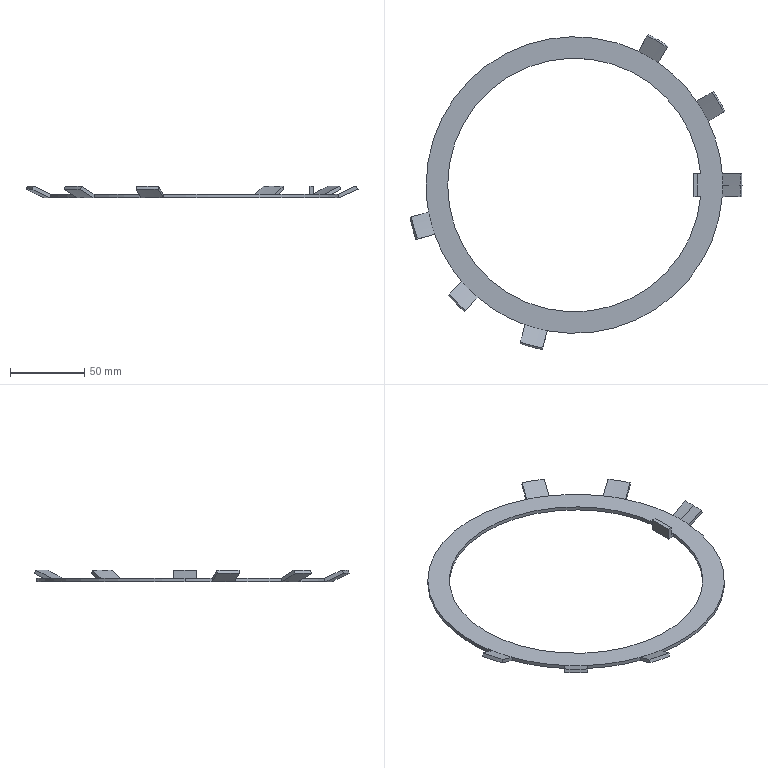Part | SolidWorks | features Boss 1, Cut 1, Revolution 1 | 1 solid | 48 faces | box 223.898 x 212.404 x 8.087 mm | volume 24578 mm3 | cone 20 | plane 19 | cylinder 9 | commonest cylinder face diameters 200 x7 171 x2
STEP:
#1=CARTESIAN_POINT('',(-100.,0.,-5.587));
#2=VERTEX_POINT('',#1);
#3=CARTESIAN_POINT('',(-98.308,-18.318,-5.587));
#4=VERTEX_POINT('',#3);
#5=CARTESIAN_POINT('',(0.,0.,-5.587));
#6=DIRECTION('',(0.,0.,1.));
#7=DIRECTION('',(1.,0.,0.));
#8=AXIS2_PLACEMENT_3D('',#5,#6,#7);
#9=CIRCLE('',#8,100.);
#10=EDGE_CURVE('',#2,#4,#9,.T.);
#11=ORIENTED_EDGE('',*,*,#10,.F.);
#12=CARTESIAN_POINT('',(-100.,0.,-8.087));
#13=VERTEX_POINT('',#12);
#14=CARTESIAN_POINT('',(-100.,0.,0.));
#15=DIRECTION('',(0.,0.,-1.));
#16=VECTOR('',#15,1000.);
#17=LINE('',#14,#16);
#18=EDGE_CURVE('',#2,#13,#17,.T.);
#19=ORIENTED_EDGE('',*,*,#18,.T.);
#20=CARTESIAN_POINT('',(-98.308,-18.318,-8.087));
#21=VERTEX_POINT('',#20);
#22=CARTESIAN_POINT('',(0.,0.,-8.087));
#23=DIRECTION('',(0.,0.,-1.));
#24=DIRECTION('',(-1.,0.,0.));
#25=AXIS2_PLACEMENT_3D('',#22,#23,#24);
#26=CIRCLE('',#25,100.);
#27=EDGE_CURVE('',#21,#13,#26,.T.);
#28=ORIENTED_EDGE('',*,*,#27,.F.);
#29=CARTESIAN_POINT('',(-98.308,-18.318,0.));
#30=DIRECTION('',(0.,0.,-1.));
#31=VECTOR('',#30,1000.);
#32=LINE('',#29,#31);
#33=EDGE_CURVE('',#4,#21,#32,.T.);
#34=ORIENTED_EDGE('',*,*,#33,.F.);
#35=EDGE_LOOP('',(#11,#19,#28,#34));
#36=FACE_OUTER_BOUND('',#35,.T.);
#37=CARTESIAN_POINT('',(0.,0.,0.));
#38=DIRECTION('',(0.,0.,-1.));
#39=DIRECTION('',(-1.,0.,0.));
#40=AXIS2_PLACEMENT_3D('',#37,#38,#39);
#41=CYLINDRICAL_SURFACE('',#40,100.);
#42=ADVANCED_FACE('',(#36),#41,.T.);
#43=CARTESIAN_POINT('',(85.148,7.75,-5.587));
#44=VERTEX_POINT('',#43);
#45=CARTESIAN_POINT('',(-85.5,0.,-5.587));
#46=VERTEX_POINT('',#45);
#47=CARTESIAN_POINT('',(0.,0.,-5.587));
#48=DIRECTION('',(0.,0.,1.));
#49=DIRECTION('',(1.,0.,0.));
#50=AXIS2_PLACEMENT_3D('',#47,#48,#49);
#51=CIRCLE('',#50,85.5);
#52=EDGE_CURVE('',#44,#46,#51,.T.);
#53=ORIENTED_EDGE('',*,*,#52,.T.);
#54=CARTESIAN_POINT('',(-85.5,0.,-8.087));
#55=VERTEX_POINT('',#54);
#56=CARTESIAN_POINT('',(-85.5,0.,0.));
#57=DIRECTION('',(0.,0.,-1.));
#58=VECTOR('',#57,1000.);
#59=LINE('',#56,#58);
#60=EDGE_CURVE('',#46,#55,#59,.T.);
#61=ORIENTED_EDGE('',*,*,#60,.T.);
#62=CARTESIAN_POINT('',(85.148,7.75,-8.087));
#63=VERTEX_POINT('',#62);
#64=CARTESIAN_POINT('',(0.,0.,-8.087));
#65=DIRECTION('',(0.,0.,-1.));
#66=DIRECTION('',(-1.,0.,0.));
#67=AXIS2_PLACEMENT_3D('',#64,#65,#66);
#68=CIRCLE('',#67,85.5);
#69=EDGE_CURVE('',#55,#63,#68,.T.);
#70=ORIENTED_EDGE('',*,*,#69,.T.);
#71=CARTESIAN_POINT('',(85.148,7.75,0.));
#72=DIRECTION('',(0.,0.,-1.));
#73=VECTOR('',#72,1000.);
#74=LINE('',#71,#73);
#75=EDGE_CURVE('',#44,#63,#74,.T.);
#76=ORIENTED_EDGE('',*,*,#75,.F.);
#77=EDGE_LOOP('',(#53,#61,#70,#76));
#78=FACE_OUTER_BOUND('',#77,.T.);
#79=CARTESIAN_POINT('',(0.,0.,0.));
#80=DIRECTION('',(0.,0.,-1.));
#81=DIRECTION('',(-1.,0.,0.));
#82=AXIS2_PLACEMENT_3D('',#79,#80,#81);
#83=CYLINDRICAL_SURFACE('',#82,85.5);
#84=ADVANCED_FACE('',(#78),#83,.F.);
#85=CARTESIAN_POINT('',(100.,0.,-5.587));
#86=VERTEX_POINT('',#85);
#87=CARTESIAN_POINT('',(99.699,7.75,-5.587));
#88=VERTEX_POINT('',#87);
#89=CARTESIAN_POINT('',(0.,0.,-5.587));
#90=DIRECTION('',(0.,0.,1.));
#91=DIRECTION('',(1.,0.,0.));
#92=AXIS2_PLACEMENT_3D('',#89,#90,#91);
#93=CIRCLE('',#92,100.);
#94=EDGE_CURVE('',#86,#88,#93,.T.);
#95=ORIENTED_EDGE('',*,*,#94,.F.);
#96=CARTESIAN_POINT('',(111.981,0.,0.));
#97=VERTEX_POINT('',#96);
#98=CARTESIAN_POINT('',(100.,0.,-5.587));
#99=DIRECTION('',(0.9063,0.,0.4226));
#100=VECTOR('',#99,1000.);
#101=LINE('',#98,#100);
#102=EDGE_CURVE('',#86,#97,#101,.T.);
#103=ORIENTED_EDGE('',*,*,#102,.T.);
#104=CARTESIAN_POINT('',(111.712,7.75,0.));
#105=VERTEX_POINT('',#104);
#106=CARTESIAN_POINT('',(0.,0.,0.));
#107=DIRECTION('',(0.,0.,1.));
#108=DIRECTION('',(1.,0.,0.));
#109=AXIS2_PLACEMENT_3D('',#106,#107,#108);
#110=CIRCLE('',#109,111.981);
#111=EDGE_CURVE('',#97,#105,#110,.T.);
#112=ORIENTED_EDGE('',*,*,#111,.T.);
#113=CARTESIAN_POINT('',(111.712,7.75,0.));
#114=CARTESIAN_POINT('',(107.708,7.75,-1.863));
#115=CARTESIAN_POINT('',(103.704,7.75,-3.725));
#116=CARTESIAN_POINT('',(99.699,7.75,-5.587));
#117=B_SPLINE_CURVE_WITH_KNOTS('',3,(#113,#114,#115,#116),.UNSPECIFIED.,.F.,.F.,(4,4),(0.01568,0.02893),.UNSPECIFIED.);
#118=EDGE_CURVE('',#105,#88,#117,.T.);
#119=ORIENTED_EDGE('',*,*,#118,.T.);
#120=EDGE_LOOP('',(#95,#103,#112,#119));
#121=FACE_OUTER_BOUND('',#120,.T.);
#122=CARTESIAN_POINT('',(0.,0.,-5.587));
#123=DIRECTION('',(0.,0.,1.));
#124=DIRECTION('',(1.,0.,0.));
#125=AXIS2_PLACEMENT_3D('',#122,#123,#124);
#126=CONICAL_SURFACE('',#125,100.,1.134);
#127=ADVANCED_FACE('',(#121),#126,.F.);
#128=CARTESIAN_POINT('',(99.699,-7.75,-8.087));
#129=VERTEX_POINT('',#128);
#130=CARTESIAN_POINT('',(100.,0.,-8.087));
#131=VERTEX_POINT('',#130);
#132=CARTESIAN_POINT('',(0.,0.,-8.087));
#133=DIRECTION('',(0.,0.,1.));
#134=DIRECTION('',(1.,0.,0.));
#135=AXIS2_PLACEMENT_3D('',#132,#133,#134);
#136=CIRCLE('',#135,100.);
#137=EDGE_CURVE('',#129,#131,#136,.T.);
#138=ORIENTED_EDGE('',*,*,#137,.T.);
#139=CARTESIAN_POINT('',(113.,0.,-2.283));
#140=VERTEX_POINT('',#139);
#141=CARTESIAN_POINT('',(113.,0.,-2.283));
#142=DIRECTION('',(0.9131,0.,0.4077));
#143=VECTOR('',#142,1000.);
#144=LINE('',#141,#143);
#145=EDGE_CURVE('',#131,#140,#144,.T.);
#146=ORIENTED_EDGE('',*,*,#145,.T.);
#147=CARTESIAN_POINT('',(112.734,-7.75,-2.283));
#148=VERTEX_POINT('',#147);
#149=CARTESIAN_POINT('',(0.,0.,-2.283));
#150=DIRECTION('',(0.,0.,1.));
#151=DIRECTION('',(1.,0.,0.));
#152=AXIS2_PLACEMENT_3D('',#149,#150,#151);
#153=CIRCLE('',#152,113.);
#154=EDGE_CURVE('',#148,#140,#153,.T.);
#155=ORIENTED_EDGE('',*,*,#154,.F.);
#156=CARTESIAN_POINT('',(112.734,-7.75,-2.283));
#157=CARTESIAN_POINT('',(108.389,-7.75,-4.218));
#158=CARTESIAN_POINT('',(104.044,-7.75,-6.153));
#159=CARTESIAN_POINT('',(99.699,-7.75,-8.087));
#160=B_SPLINE_CURVE_WITH_KNOTS('',3,(#156,#157,#158,#159),.UNSPECIFIED.,.F.,.F.,(4,4),(0.01634,0.03061),.UNSPECIFIED.);
#161=EDGE_CURVE('',#148,#129,#160,.T.);
#162=ORIENTED_EDGE('',*,*,#161,.T.);
#163=EDGE_LOOP('',(#138,#146,#155,#162));
#164=FACE_OUTER_BOUND('',#163,.T.);
#165=CARTESIAN_POINT('',(0.,0.,-2.283));
#166=DIRECTION('',(0.,0.,1.));
#167=DIRECTION('',(1.,0.,0.));
#168=AXIS2_PLACEMENT_3D('',#165,#166,#167);
#169=CONICAL_SURFACE('',#168,113.,1.151);
#170=ADVANCED_FACE('',(#164),#169,.T.);
#171=CARTESIAN_POINT('',(90.217,43.138,-5.587));
#172=VERTEX_POINT('',#171);
#173=CARTESIAN_POINT('',(0.,0.,-5.587));
#174=DIRECTION('',(0.,0.,1.));
#175=DIRECTION('',(1.,0.,0.));
#176=AXIS2_PLACEMENT_3D('',#173,#174,#175);
#177=CIRCLE('',#176,100.);
#178=EDGE_CURVE('',#88,#172,#177,.T.);
#179=ORIENTED_EDGE('',*,*,#178,.T.);
#180=CARTESIAN_POINT('',(82.467,56.561,-5.587));
#181=VERTEX_POINT('',#180);
#182=CARTESIAN_POINT('',(0.,0.,-5.587));
#183=DIRECTION('',(0.,0.,1.));
#184=DIRECTION('',(1.,0.,0.));
#185=AXIS2_PLACEMENT_3D('',#182,#183,#184);
#186=CIRCLE('',#185,100.);
#187=EDGE_CURVE('',#172,#181,#186,.T.);
#188=ORIENTED_EDGE('',*,*,#187,.T.);
#189=CARTESIAN_POINT('',(56.561,82.467,-5.587));
#190=VERTEX_POINT('',#189);
#191=CARTESIAN_POINT('',(0.,0.,-5.587));
#192=DIRECTION('',(0.,0.,1.));
#193=DIRECTION('',(1.,0.,0.));
#194=AXIS2_PLACEMENT_3D('',#191,#192,#193);
#195=CIRCLE('',#194,100.);
#196=EDGE_CURVE('',#181,#190,#195,.T.);
#197=ORIENTED_EDGE('',*,*,#196,.T.);
#198=CARTESIAN_POINT('',(43.138,90.217,-5.587));
#199=VERTEX_POINT('',#198);
#200=CARTESIAN_POINT('',(0.,0.,-5.587));
#201=DIRECTION('',(0.,0.,1.));
#202=DIRECTION('',(1.,0.,0.));
#203=AXIS2_PLACEMENT_3D('',#200,#201,#202);
#204=CIRCLE('',#203,100.);
#205=EDGE_CURVE('',#190,#199,#204,.T.);
#206=ORIENTED_EDGE('',*,*,#205,.T.);
#207=CARTESIAN_POINT('',(0.,0.,-5.587));
#208=DIRECTION('',(0.,0.,1.));
#209=DIRECTION('',(1.,0.,0.));
#210=AXIS2_PLACEMENT_3D('',#207,#208,#209);
#211=CIRCLE('',#210,100.);
#212=EDGE_CURVE('',#199,#2,#211,.T.);
#213=ORIENTED_EDGE('',*,*,#212,.T.);
#214=ORIENTED_EDGE('',*,*,#10,.T.);
#215=CARTESIAN_POINT('',(-94.296,-33.29,-5.587));
#216=VERTEX_POINT('',#215);
#217=CARTESIAN_POINT('',(0.,0.,-5.587));
#218=DIRECTION('',(0.,0.,1.));
#219=DIRECTION('',(1.,0.,0.));
#220=AXIS2_PLACEMENT_3D('',#217,#218,#219);
#221=CIRCLE('',#220,100.);
#222=EDGE_CURVE('',#4,#216,#221,.T.);
#223=ORIENTED_EDGE('',*,*,#222,.T.);
#224=CARTESIAN_POINT('',(-75.978,-65.018,-5.587));
#225=VERTEX_POINT('',#224);
#226=CARTESIAN_POINT('',(0.,0.,-5.587));
#227=DIRECTION('',(0.,0.,1.));
#228=DIRECTION('',(1.,0.,0.));
#229=AXIS2_PLACEMENT_3D('',#226,#227,#228);
#230=CIRCLE('',#229,100.);
#231=EDGE_CURVE('',#216,#225,#230,.T.);
#232=ORIENTED_EDGE('',*,*,#231,.T.);
#233=CARTESIAN_POINT('',(-65.018,-75.978,-5.587));
#234=VERTEX_POINT('',#233);
#235=CARTESIAN_POINT('',(0.,0.,-5.587));
#236=DIRECTION('',(0.,0.,1.));
#237=DIRECTION('',(1.,0.,0.));
#238=AXIS2_PLACEMENT_3D('',#235,#236,#237);
#239=CIRCLE('',#238,100.);
#240=EDGE_CURVE('',#225,#234,#239,.T.);
#241=ORIENTED_EDGE('',*,*,#240,.T.);
#242=CARTESIAN_POINT('',(-33.29,-94.296,-5.587));
#243=VERTEX_POINT('',#242);
#244=CARTESIAN_POINT('',(0.,0.,-5.587));
#245=DIRECTION('',(0.,0.,1.));
#246=DIRECTION('',(1.,0.,0.));
#247=AXIS2_PLACEMENT_3D('',#244,#245,#246);
#248=CIRCLE('',#247,100.);
#249=EDGE_CURVE('',#234,#243,#248,.T.);
#250=ORIENTED_EDGE('',*,*,#249,.T.);
#251=CARTESIAN_POINT('',(-18.318,-98.308,-5.587));
#252=VERTEX_POINT('',#251);
#253=CARTESIAN_POINT('',(0.,0.,-5.587));
#254=DIRECTION('',(0.,0.,1.));
#255=DIRECTION('',(1.,0.,0.));
#256=AXIS2_PLACEMENT_3D('',#253,#254,#255);
#257=CIRCLE('',#256,100.);
#258=EDGE_CURVE('',#243,#252,#257,.T.);
#259=ORIENTED_EDGE('',*,*,#258,.T.);
#260=CARTESIAN_POINT('',(99.699,-7.75,-5.587));
#261=VERTEX_POINT('',#260);
#262=CARTESIAN_POINT('',(0.,0.,-5.587));
#263=DIRECTION('',(0.,0.,1.));
#264=DIRECTION('',(1.,0.,0.));
#265=AXIS2_PLACEMENT_3D('',#262,#263,#264);
#266=CIRCLE('',#265,100.);
#267=EDGE_CURVE('',#252,#261,#266,.T.);
#268=ORIENTED_EDGE('',*,*,#267,.T.);
#269=CARTESIAN_POINT('',(0.,0.,-5.587));
#270=DIRECTION('',(0.,0.,1.));
#271=DIRECTION('',(1.,0.,0.));
#272=AXIS2_PLACEMENT_3D('',#269,#270,#271);
#273=CIRCLE('',#272,100.);
#274=EDGE_CURVE('',#261,#86,#273,.T.);
#275=ORIENTED_EDGE('',*,*,#274,.T.);
#276=ORIENTED_EDGE('',*,*,#94,.T.);
#277=EDGE_LOOP('',(#179,#188,#197,#206,#213,#214,#223,#232,#241,#250,#259,#268,#275,#276));
#278=FACE_OUTER_BOUND('',#277,.T.);
#279=CARTESIAN_POINT('',(83.,7.75,-5.587));
#280=VERTEX_POINT('',#279);
#281=CARTESIAN_POINT('',(0.,7.75,-5.587));
#282=DIRECTION('',(1.,0.,0.));
#283=VECTOR('',#282,1000.);
#284=LINE('',#281,#283);
#285=EDGE_CURVE('',#280,#44,#284,.T.);
#286=ORIENTED_EDGE('',*,*,#285,.F.);
#287=CARTESIAN_POINT('',(83.,-7.75,-5.587));
#288=VERTEX_POINT('',#287);
#289=CARTESIAN_POINT('',(83.,-7.75,-5.587));
#290=DIRECTION('',(0.,-1.,0.));
#291=VECTOR('',#290,1000.);
#292=LINE('',#289,#291);
#293=EDGE_CURVE('',#280,#288,#292,.T.);
#294=ORIENTED_EDGE('',*,*,#293,.T.);
#295=CARTESIAN_POINT('',(85.148,-7.75,-5.587));
#296=VERTEX_POINT('',#295);
#297=CARTESIAN_POINT('',(0.,-7.75,-5.587));
#298=DIRECTION('',(-1.,0.,0.));
#299=VECTOR('',#298,1000.);
#300=LINE('',#297,#299);
#301=EDGE_CURVE('',#296,#288,#300,.T.);
#302=ORIENTED_EDGE('',*,*,#301,.F.);
#303=CARTESIAN_POINT('',(0.,0.,-5.587));
#304=DIRECTION('',(0.,0.,1.));
#305=DIRECTION('',(1.,0.,0.));
#306=AXIS2_PLACEMENT_3D('',#303,#304,#305);
#307=CIRCLE('',#306,85.5);
#308=EDGE_CURVE('',#46,#296,#307,.T.);
#309=ORIENTED_EDGE('',*,*,#308,.F.);
#310=ORIENTED_EDGE('',*,*,#52,.F.);
#311=EDGE_LOOP('',(#286,#294,#302,#309,#310));
#312=FACE_BOUND('',#311,.T.);
#313=CARTESIAN_POINT('',(0.,-100.,-5.587));
#314=DIRECTION('',(0.,0.,1.));
#315=DIRECTION('',(1.,0.,0.));
#316=AXIS2_PLACEMENT_3D('',#313,#314,#315);
#317=PLANE('',#316);
#318=ADVANCED_FACE('',(#278,#312),#317,.T.);
#319=ORIENTED_EDGE('',*,*,#145,.F.);
#320=CARTESIAN_POINT('',(99.699,7.75,-8.087));
#321=VERTEX_POINT('',#320);
#322=CARTESIAN_POINT('',(0.,0.,-8.087));
#323=DIRECTION('',(0.,0.,1.));
#324=DIRECTION('',(1.,0.,0.));
#325=AXIS2_PLACEMENT_3D('',#322,#323,#324);
#326=CIRCLE('',#325,100.);
#327=EDGE_CURVE('',#131,#321,#326,.T.);
#328=ORIENTED_EDGE('',*,*,#327,.T.);
#329=CARTESIAN_POINT('',(112.734,7.75,-2.283));
#330=VERTEX_POINT('',#329);
#331=CARTESIAN_POINT('',(99.699,7.75,-8.087));
#332=CARTESIAN_POINT('',(104.044,7.75,-6.153));
#333=CARTESIAN_POINT('',(108.389,7.75,-4.218));
#334=CARTESIAN_POINT('',(112.734,7.75,-2.283));
#335=B_SPLINE_CURVE_WITH_KNOTS('',3,(#331,#332,#333,#334),.UNSPECIFIED.,.F.,.F.,(4,4),(0.02645,0.04072),.UNSPECIFIED.);
#336=EDGE_CURVE('',#321,#330,#335,.T.);
#337=ORIENTED_EDGE('',*,*,#336,.T.);
#338=CARTESIAN_POINT('',(0.,0.,-2.283));
#339=DIRECTION('',(0.,0.,1.));
#340=DIRECTION('',(1.,0.,0.));
#341=AXIS2_PLACEMENT_3D('',#338,#339,#340);
#342=CIRCLE('',#341,113.);
#343=EDGE_CURVE('',#140,#330,#342,.T.);
#344=ORIENTED_EDGE('',*,*,#343,.F.);
#345=EDGE_LOOP('',(#319,#328,#337,#344));
#346=FACE_OUTER_BOUND('',#345,.T.);
#347=CARTESIAN_POINT('',(0.,0.,-2.283));
#348=DIRECTION('',(0.,0.,1.));
#349=DIRECTION('',(1.,0.,0.));
#350=AXIS2_PLACEMENT_3D('',#347,#348,#349);
#351=CONICAL_SURFACE('',#350,113.,1.151);
#352=ADVANCED_FACE('',(#346),#351,.T.);
#353=CARTESIAN_POINT('',(101.505,49.655,-2.283));
#354=VERTEX_POINT('',#353);
#355=CARTESIAN_POINT('',(93.755,63.079,-2.283));
#356=VERTEX_POINT('',#355);
#357=CARTESIAN_POINT('',(0.,0.,-2.283));
#358=DIRECTION('',(0.,0.,1.));
#359=DIRECTION('',(1.,0.,0.));
#360=AXIS2_PLACEMENT_3D('',#357,#358,#359);
#361=CIRCLE('',#360,113.);
#362=EDGE_CURVE('',#354,#356,#361,.T.);
#363=ORIENTED_EDGE('',*,*,#362,.F.);
#364=CARTESIAN_POINT('',(90.217,43.138,-8.087));
#365=VERTEX_POINT('',#364);
#366=CARTESIAN_POINT('',(101.505,49.655,-2.283));
#367=CARTESIAN_POINT('',(97.743,47.483,-4.218));
#368=CARTESIAN_POINT('',(93.98,45.31,-6.153));
#369=CARTESIAN_POINT('',(90.217,43.138,-8.087));
#370=B_SPLINE_CURVE_WITH_KNOTS('',3,(#366,#367,#368,#369),.UNSPECIFIED.,.F.,.F.,(4,4),(0.000000253,0.01427),.UNSPECIFIED.);
#371=EDGE_CURVE('',#354,#365,#370,.T.);
#372=ORIENTED_EDGE('',*,*,#371,.T.);
#373=CARTESIAN_POINT('',(82.467,56.561,-8.087));
#374=VERTEX_POINT('',#373);
#375=CARTESIAN_POINT('',(0.,0.,-8.087));
#376=DIRECTION('',(0.,0.,1.));
#377=DIRECTION('',(1.,0.,0.));
#378=AXIS2_PLACEMENT_3D('',#375,#376,#377);
#379=CIRCLE('',#378,100.);
#380=EDGE_CURVE('',#365,#374,#379,.T.);
#381=ORIENTED_EDGE('',*,*,#380,.T.);
#382=CARTESIAN_POINT('',(82.467,56.561,-8.087));
#383=CARTESIAN_POINT('',(86.23,58.734,-6.153));
#384=CARTESIAN_POINT('',(89.993,60.906,-4.218));
#385=CARTESIAN_POINT('',(93.755,63.079,-2.283));
#386=B_SPLINE_CURVE_WITH_KNOTS('',3,(#382,#383,#384,#385),.UNSPECIFIED.,.F.,.F.,(4,4),(0.000000253,0.01427),.UNSPECIFIED.);
#387=EDGE_CURVE('',#374,#356,#386,.T.);
#388=ORIENTED_EDGE('',*,*,#387,.T.);
#389=EDGE_LOOP('',(#363,#372,#381,#388));
#390=FACE_OUTER_BOUND('',#389,.T.);
#391=CARTESIAN_POINT('',(0.,0.,-2.283));
#392=DIRECTION('',(0.,0.,1.));
#393=DIRECTION('',(1.,0.,0.));
#394=AXIS2_PLACEMENT_3D('',#391,#392,#393);
#395=CONICAL_SURFACE('',#394,113.,1.151);
#396=ADVANCED_FACE('',(#390),#395,.T.);
#397=CARTESIAN_POINT('',(63.079,93.755,-2.283));
#398=VERTEX_POINT('',#397);
#399=CARTESIAN_POINT('',(49.655,101.505,-2.283));
#400=VERTEX_POINT('',#399);
#401=CARTESIAN_POINT('',(0.,0.,-2.283));
#402=DIRECTION('',(0.,0.,1.));
#403=DIRECTION('',(1.,0.,0.));
#404=AXIS2_PLACEMENT_3D('',#401,#402,#403);
#405=CIRCLE('',#404,113.);
#406=EDGE_CURVE('',#398,#400,#405,.T.);
#407=ORIENTED_EDGE('',*,*,#406,.F.);
#408=CARTESIAN_POINT('',(56.561,82.467,-8.087));
#409=VERTEX_POINT('',#408);
#410=CARTESIAN_POINT('',(63.079,93.755,-2.283));
#411=CARTESIAN_POINT('',(60.906,89.993,-4.218));
#412=CARTESIAN_POINT('',(58.734,86.23,-6.153));
#413=CARTESIAN_POINT('',(56.561,82.467,-8.087));
#414=B_SPLINE_CURVE_WITH_KNOTS('',3,(#410,#411,#412,#413),.UNSPECIFIED.,.F.,.F.,(4,4),(0.000000253,0.01427),.UNSPECIFIED.);
#415=EDGE_CURVE('',#398,#409,#414,.T.);
#416=ORIENTED_EDGE('',*,*,#415,.T.);
#417=CARTESIAN_POINT('',(43.138,90.217,-8.087));
#418=VERTEX_POINT('',#417);
#419=CARTESIAN_POINT('',(0.,0.,-8.087));
#420=DIRECTION('',(0.,0.,1.));
#421=DIRECTION('',(1.,0.,0.));
#422=AXIS2_PLACEMENT_3D('',#419,#420,#421);
#423=CIRCLE('',#422,100.);
#424=EDGE_CURVE('',#409,#418,#423,.T.);
#425=ORIENTED_EDGE('',*,*,#424,.T.);
#426=CARTESIAN_POINT('',(43.138,90.217,-8.087));
#427=CARTESIAN_POINT('',(45.31,93.98,-6.153));
#428=CARTESIAN_POINT('',(47.483,97.743,-4.218));
#429=CARTESIAN_POINT('',(49.655,101.505,-2.283));
#430=B_SPLINE_CURVE_WITH_KNOTS('',3,(#426,#427,#428,#429),.UNSPECIFIED.,.F.,.F.,(4,4),(0.000000253,0.01427),.UNSPECIFIED.);
#431=EDGE_CURVE('',#418,#400,#430,.T.);
#432=ORIENTED_EDGE('',*,*,#431,.T.);
#433=EDGE_LOOP('',(#407,#416,#425,#432));
#434=FACE_OUTER_BOUND('',#433,.T.);
#435=CARTESIAN_POINT('',(0.,0.,-2.283));
#436=DIRECTION('',(0.,0.,1.));
#437=DIRECTION('',(1.,0.,0.));
#438=AXIS2_PLACEMENT_3D('',#435,#436,#437);
#439=CONICAL_SURFACE('',#438,113.,1.151);
#440=ADVANCED_FACE('',(#434),#439,.T.);
#441=CARTESIAN_POINT('',(-110.898,-21.692,-2.283));
#442=VERTEX_POINT('',#441);
#443=CARTESIAN_POINT('',(-106.887,-36.664,-2.283));
#444=VERTEX_POINT('',#443);
#445=CARTESIAN_POINT('',(0.,0.,-2.283));
#446=DIRECTION('',(0.,0.,1.));
#447=DIRECTION('',(1.,0.,0.));
#448=AXIS2_PLACEMENT_3D('',#445,#446,#447);
#449=CIRCLE('',#448,113.);
#450=EDGE_CURVE('',#442,#444,#449,.T.);
#451=ORIENTED_EDGE('',*,*,#450,.F.);
#452=CARTESIAN_POINT('',(-110.898,-21.692,-2.283));
#453=CARTESIAN_POINT('',(-106.702,-20.567,-4.218));
#454=CARTESIAN_POINT('',(-102.505,-19.443,-6.153));
#455=CARTESIAN_POINT('',(-98.308,-18.318,-8.087));
#456=B_SPLINE_CURVE_WITH_KNOTS('',3,(#452,#453,#454,#455),.UNSPECIFIED.,.F.,.F.,(4,4),(0.000000227,0.01427),.UNSPECIFIED.);
#457=EDGE_CURVE('',#442,#21,#456,.T.);
#458=ORIENTED_EDGE('',*,*,#457,.T.);
#459=CARTESIAN_POINT('',(-94.296,-33.29,-8.087));
#460=VERTEX_POINT('',#459);
#461=CARTESIAN_POINT('',(0.,0.,-8.087));
#462=DIRECTION('',(0.,0.,1.));
#463=DIRECTION('',(1.,0.,0.));
#464=AXIS2_PLACEMENT_3D('',#461,#462,#463);
#465=CIRCLE('',#464,100.);
#466=EDGE_CURVE('',#21,#460,#465,.T.);
#467=ORIENTED_EDGE('',*,*,#466,.T.);
#468=CARTESIAN_POINT('',(-94.296,-33.29,-8.087));
#469=CARTESIAN_POINT('',(-98.493,-34.415,-6.153));
#470=CARTESIAN_POINT('',(-102.69,-35.539,-4.218));
#471=CARTESIAN_POINT('',(-106.887,-36.664,-2.283));
#472=B_SPLINE_CURVE_WITH_KNOTS('',3,(#468,#469,#470,#471),.UNSPECIFIED.,.F.,.F.,(4,4),(0.000000227,0.01427),.UNSPECIFIED.);
#473=EDGE_CURVE('',#460,#444,#472,.T.);
#474=ORIENTED_EDGE('',*,*,#473,.T.);
#475=EDGE_LOOP('',(#451,#458,#467,#474));
#476=FACE_OUTER_BOUND('',#475,.T.);
#477=CARTESIAN_POINT('',(0.,0.,-2.283));
#478=DIRECTION('',(0.,0.,1.));
#479=DIRECTION('',(1.,0.,0.));
#480=AXIS2_PLACEMENT_3D('',#477,#478,#479);
#481=CONICAL_SURFACE('',#480,113.,1.151);
#482=ADVANCED_FACE('',(#476),#481,.T.);
#483=CARTESIAN_POINT('',(-85.195,-74.235,-2.283));
#484=VERTEX_POINT('',#483);
#485=CARTESIAN_POINT('',(-74.235,-85.195,-2.283));
#486=VERTEX_POINT('',#485);
#487=CARTESIAN_POINT('',(0.,0.,-2.283));
#488=DIRECTION('',(0.,0.,1.));
#489=DIRECTION('',(1.,0.,0.));
#490=AXIS2_PLACEMENT_3D('',#487,#488,#489);
#491=CIRCLE('',#490,113.);
#492=EDGE_CURVE('',#484,#486,#491,.T.);
#493=ORIENTED_EDGE('',*,*,#492,.F.);
#494=CARTESIAN_POINT('',(-75.978,-65.018,-8.087));
#495=VERTEX_POINT('',#494);
#496=CARTESIAN_POINT('',(-85.195,-74.235,-2.283));
#497=CARTESIAN_POINT('',(-82.123,-71.163,-4.218));
#498=CARTESIAN_POINT('',(-79.051,-68.09,-6.153));
#499=CARTESIAN_POINT('',(-75.978,-65.018,-8.087));
#500=B_SPLINE_CURVE_WITH_KNOTS('',3,(#496,#497,#498,#499),.UNSPECIFIED.,.F.,.F.,(4,4),(0.00000031,0.01427),.UNSPECIFIED.);
#501=EDGE_CURVE('',#484,#495,#500,.T.);
#502=ORIENTED_EDGE('',*,*,#501,.T.);
#503=CARTESIAN_POINT('',(-65.018,-75.978,-8.087));
#504=VERTEX_POINT('',#503);
#505=CARTESIAN_POINT('',(0.,0.,-8.087));
#506=DIRECTION('',(0.,0.,1.));
#507=DIRECTION('',(1.,0.,0.));
#508=AXIS2_PLACEMENT_3D('',#505,#506,#507);
#509=CIRCLE('',#508,100.);
#510=EDGE_CURVE('',#495,#504,#509,.T.);
#511=ORIENTED_EDGE('',*,*,#510,.T.);
#512=CARTESIAN_POINT('',(-65.018,-75.978,-8.087));
#513=CARTESIAN_POINT('',(-68.09,-79.051,-6.153));
#514=CARTESIAN_POINT('',(-71.163,-82.123,-4.218));
#515=CARTESIAN_POINT('',(-74.235,-85.195,-2.283));
#516=B_SPLINE_CURVE_WITH_KNOTS('',3,(#512,#513,#514,#515),.UNSPECIFIED.,.F.,.F.,(4,4),(0.00000031,0.01427),.UNSPECIFIED.);
#517=EDGE_CURVE('',#504,#486,#516,.T.);
#518=ORIENTED_EDGE('',*,*,#517,.T.);
#519=EDGE_LOOP('',(#493,#502,#511,#518));
#520=FACE_OUTER_BOUND('',#519,.T.);
#521=CARTESIAN_POINT('',(0.,0.,-2.283));
#522=DIRECTION('',(0.,0.,1.));
#523=DIRECTION('',(1.,0.,0.));
#524=AXIS2_PLACEMENT_3D('',#521,#522,#523);
#525=CONICAL_SURFACE('',#524,113.,1.151);
#526=ADVANCED_FACE('',(#520),#525,.T.);
#527=CARTESIAN_POINT('',(-36.664,-106.887,-2.283));
#528=VERTEX_POINT('',#527);
#529=CARTESIAN_POINT('',(-21.692,-110.898,-2.283));
#530=VERTEX_POINT('',#529);
#531=CARTESIAN_POINT('',(0.,0.,-2.283));
#532=DIRECTION('',(0.,0.,1.));
#533=DIRECTION('',(1.,0.,0.));
#534=AXIS2_PLACEMENT_3D('',#531,#532,#533);
#535=CIRCLE('',#534,113.);
#536=EDGE_CURVE('',#528,#530,#535,.T.);
#537=ORIENTED_EDGE('',*,*,#536,.F.);
#538=CARTESIAN_POINT('',(-33.29,-94.296,-8.087));
#539=VERTEX_POINT('',#538);
#540=CARTESIAN_POINT('',(-36.664,-106.887,-2.283));
#541=CARTESIAN_POINT('',(-35.539,-102.69,-4.218));
#542=CARTESIAN_POINT('',(-34.415,-98.493,-6.153));
#543=CARTESIAN_POINT('',(-33.29,-94.296,-8.087));
#544=B_SPLINE_CURVE_WITH_KNOTS('',3,(#540,#541,#542,#543),.UNSPECIFIED.,.F.,.F.,(4,4),(0.000000227,0.01427),.UNSPECIFIED.);
#545=EDGE_CURVE('',#528,#539,#544,.T.);
#546=ORIENTED_EDGE('',*,*,#545,.T.);
#547=CARTESIAN_POINT('',(-18.318,-98.308,-8.087));
#548=VERTEX_POINT('',#547);
#549=CARTESIAN_POINT('',(0.,0.,-8.087));
#550=DIRECTION('',(0.,0.,1.));
#551=DIRECTION('',(1.,0.,0.));
#552=AXIS2_PLACEMENT_3D('',#549,#550,#551);
#553=CIRCLE('',#552,100.);
#554=EDGE_CURVE('',#539,#548,#553,.T.);
#555=ORIENTED_EDGE('',*,*,#554,.T.);
#556=CARTESIAN_POINT('',(-18.318,-98.308,-8.087));
#557=CARTESIAN_POINT('',(-19.443,-102.505,-6.153));
#558=CARTESIAN_POINT('',(-20.567,-106.702,-4.218));
#559=CARTESIAN_POINT('',(-21.692,-110.898,-2.283));
#560=B_SPLINE_CURVE_WITH_KNOTS('',3,(#556,#557,#558,#559),.UNSPECIFIED.,.F.,.F.,(4,4),(0.000000227,0.01427),.UNSPECIFIED.);
#561=EDGE_CURVE('',#548,#530,#560,.T.);
#562=ORIENTED_EDGE('',*,*,#561,.T.);
#563=EDGE_LOOP('',(#537,#546,#555,#562));
#564=FACE_OUTER_BOUND('',#563,.T.);
#565=CARTESIAN_POINT('',(0.,0.,-2.283));
#566=DIRECTION('',(0.,0.,1.));
#567=DIRECTION('',(1.,0.,0.));
#568=AXIS2_PLACEMENT_3D('',#565,#566,#567);
#569=CONICAL_SURFACE('',#568,113.,1.151);
#570=ADVANCED_FACE('',(#564),#569,.T.);
#571=CARTESIAN_POINT('',(111.712,-7.75,0.));
#572=VERTEX_POINT('',#571);
#573=CARTESIAN_POINT('',(0.,0.,0.));
#574=DIRECTION('',(0.,0.,1.));
#575=DIRECTION('',(1.,0.,0.));
#576=AXIS2_PLACEMENT_3D('',#573,#574,#575);
#577=CIRCLE('',#576,111.981);
#578=EDGE_CURVE('',#572,#97,#577,.T.);
#579=ORIENTED_EDGE('',*,*,#578,.F.);
#580=CARTESIAN_POINT('',(111.712,-7.75,0.));
#581=CARTESIAN_POINT('',(111.82,-7.75,-0.2414));
#582=CARTESIAN_POINT('',(111.928,-7.75,-0.4829));
#583=CARTESIAN_POINT('',(112.036,-7.75,-0.7243));
#584=CARTESIAN_POINT('',(112.269,-7.75,-1.244));
#585=CARTESIAN_POINT('',(112.501,-7.75,-1.763));
#586=CARTESIAN_POINT('',(112.734,-7.75,-2.283));
#587=B_SPLINE_CURVE_WITH_KNOTS('',3,(#580,#581,#582,#583,#584,#585,#586),.UNSPECIFIED.,.F.,.F.,(4,3,4),(0.02365,0.02444,0.02615),.UNSPECIFIED.);
#588=EDGE_CURVE('',#572,#148,#587,.T.);
#589=ORIENTED_EDGE('',*,*,#588,.T.);
#590=ORIENTED_EDGE('',*,*,#154,.T.);
#591=ORIENTED_EDGE('',*,*,#343,.T.);
#592=CARTESIAN_POINT('',(112.734,7.75,-2.283));
#593=CARTESIAN_POINT('',(112.501,7.75,-1.763));
#594=CARTESIAN_POINT('',(112.269,7.75,-1.244));
#595=CARTESIAN_POINT('',(112.036,7.75,-0.7243));
#596=CARTESIAN_POINT('',(111.928,7.75,-0.4829));
#597=CARTESIAN_POINT('',(111.82,7.75,-0.2414));
#598=CARTESIAN_POINT('',(111.712,7.75,0.));
#599=B_SPLINE_CURVE_WITH_KNOTS('',3,(#592,#593,#594,#595,#596,#597,#598),.UNSPECIFIED.,.F.,.F.,(4,3,4),(0.02273,0.02444,0.02524),.UNSPECIFIED.);
#600=EDGE_CURVE('',#330,#105,#599,.T.);
#601=ORIENTED_EDGE('',*,*,#600,.T.);
#602=ORIENTED_EDGE('',*,*,#111,.F.);
#603=EDGE_LOOP('',(#579,#589,#590,#591,#601,#602));
#604=FACE_OUTER_BOUND('',#603,.T.);
#605=CARTESIAN_POINT('',(0.,0.,0.));
#606=DIRECTION('',(0.,0.,-1.));
#607=DIRECTION('',(-1.,0.,0.));
#608=AXIS2_PLACEMENT_3D('',#605,#606,#607);
#609=CONICAL_SURFACE('',#608,111.981,0.4199);
#610=ADVANCED_FACE('',(#604),#609,.T.);
#611=CARTESIAN_POINT('',(100.621,49.144,0.));
#612=VERTEX_POINT('',#611);
#613=CARTESIAN_POINT('',(92.871,62.568,0.));
#614=VERTEX_POINT('',#613);
#615=CARTESIAN_POINT('',(0.,0.,0.));
#616=DIRECTION('',(0.,0.,1.));
#617=DIRECTION('',(1.,0.,0.));
#618=AXIS2_PLACEMENT_3D('',#615,#616,#617);
#619=CIRCLE('',#618,111.981);
#620=EDGE_CURVE('',#612,#614,#619,.T.);
#621=ORIENTED_EDGE('',*,*,#620,.F.);
#622=CARTESIAN_POINT('',(100.621,49.144,0.));
#623=CARTESIAN_POINT('',(100.916,49.315,-0.7609));
#624=CARTESIAN_POINT('',(101.211,49.485,-1.522));
#625=CARTESIAN_POINT('',(101.505,49.655,-2.283));
#626=B_SPLINE_CURVE_WITH_KNOTS('',3,(#622,#623,#624,#625),.UNSPECIFIED.,.F.,.F.,(4,4),(0.000000219,0.002501),.UNSPECIFIED.);
#627=EDGE_CURVE('',#612,#354,#626,.T.);
#628=ORIENTED_EDGE('',*,*,#627,.T.);
#629=ORIENTED_EDGE('',*,*,#362,.T.);
#630=CARTESIAN_POINT('',(93.755,63.079,-2.283));
#631=CARTESIAN_POINT('',(93.461,62.908,-1.522));
#632=CARTESIAN_POINT('',(93.166,62.738,-0.7609));
#633=CARTESIAN_POINT('',(92.871,62.568,0.));
#634=B_SPLINE_CURVE_WITH_KNOTS('',3,(#630,#631,#632,#633),.UNSPECIFIED.,.F.,.F.,(4,4),(0.000000219,0.002501),.UNSPECIFIED.);
#635=EDGE_CURVE('',#356,#614,#634,.T.);
#636=ORIENTED_EDGE('',*,*,#635,.T.);
#637=EDGE_LOOP('',(#621,#628,#629,#636));
#638=FACE_OUTER_BOUND('',#637,.T.);
#639=CARTESIAN_POINT('',(0.,0.,0.));
#640=DIRECTION('',(0.,0.,-1.));
#641=DIRECTION('',(-1.,0.,0.));
#642=AXIS2_PLACEMENT_3D('',#639,#640,#641);
#643=CONICAL_SURFACE('',#642,111.981,0.4199);
#644=ADVANCED_FACE('',(#638),#643,.T.);
#645=CARTESIAN_POINT('',(62.568,92.871,0.));
#646=VERTEX_POINT('',#645);
#647=CARTESIAN_POINT('',(49.144,100.621,0.));
#648=VERTEX_POINT('',#647);
#649=CARTESIAN_POINT('',(0.,0.,0.));
#650=DIRECTION('',(0.,0.,1.));
#651=DIRECTION('',(1.,0.,0.));
#652=AXIS2_PLACEMENT_3D('',#649,#650,#651);
#653=CIRCLE('',#652,111.981);
#654=EDGE_CURVE('',#646,#648,#653,.T.);
#655=ORIENTED_EDGE('',*,*,#654,.F.);
#656=CARTESIAN_POINT('',(62.568,92.871,0.));
#657=CARTESIAN_POINT('',(62.738,93.166,-0.7609));
#658=CARTESIAN_POINT('',(62.908,93.461,-1.522));
#659=CARTESIAN_POINT('',(63.079,93.755,-2.283));
#660=B_SPLINE_CURVE_WITH_KNOTS('',3,(#656,#657,#658,#659),.UNSPECIFIED.,.F.,.F.,(4,4),(0.000000219,0.002501),.UNSPECIFIED.);
#661=EDGE_CURVE('',#646,#398,#660,.T.);
#662=ORIENTED_EDGE('',*,*,#661,.T.);
#663=ORIENTED_EDGE('',*,*,#406,.T.);
#664=CARTESIAN_POINT('',(49.655,101.505,-2.283));
#665=CARTESIAN_POINT('',(49.485,101.211,-1.522));
#666=CARTESIAN_POINT('',(49.315,100.916,-0.7609));
#667=CARTESIAN_POINT('',(49.144,100.621,0.));
#668=B_SPLINE_CURVE_WITH_KNOTS('',3,(#664,#665,#666,#667),.UNSPECIFIED.,.F.,.F.,(4,4),(0.000000219,0.002501),.UNSPECIFIED.);
#669=EDGE_CURVE('',#400,#648,#668,.T.);
#670=ORIENTED_EDGE('',*,*,#669,.T.);
#671=EDGE_LOOP('',(#655,#662,#663,#670));
#672=FACE_OUTER_BOUND('',#671,.T.);
#673=CARTESIAN_POINT('',(0.,0.,0.));
#674=DIRECTION('',(0.,0.,-1.));
#675=DIRECTION('',(-1.,0.,0.));
#676=AXIS2_PLACEMENT_3D('',#673,#674,#675);
#677=CONICAL_SURFACE('',#676,111.981,0.4199);
#678=ADVANCED_FACE('',(#672),#677,.T.);
#679=CARTESIAN_POINT('',(-109.912,-21.427,0.));
#680=VERTEX_POINT('',#679);
#681=CARTESIAN_POINT('',(-105.9,-36.399,0.));
#682=VERTEX_POINT('',#681);
#683=CARTESIAN_POINT('',(0.,0.,0.));
#684=DIRECTION('',(0.,0.,1.));
#685=DIRECTION('',(1.,0.,0.));
#686=AXIS2_PLACEMENT_3D('',#683,#684,#685);
#687=CIRCLE('',#686,111.981);
#688=EDGE_CURVE('',#680,#682,#687,.T.);
#689=ORIENTED_EDGE('',*,*,#688,.F.);
#690=CARTESIAN_POINT('',(-109.912,-21.427,0.));
#691=CARTESIAN_POINT('',(-110.241,-21.515,-0.7609));
#692=CARTESIAN_POINT('',(-110.57,-21.604,-1.522));
#693=CARTESIAN_POINT('',(-110.898,-21.692,-2.283));
#694=B_SPLINE_CURVE_WITH_KNOTS('',3,(#690,#691,#692,#693),.UNSPECIFIED.,.F.,.F.,(4,4),(0.000000219,0.002501),.UNSPECIFIED.);
#695=EDGE_CURVE('',#680,#442,#694,.T.);
#696=ORIENTED_EDGE('',*,*,#695,.T.);
#697=ORIENTED_EDGE('',*,*,#450,.T.);
#698=CARTESIAN_POINT('',(-106.887,-36.664,-2.283));
#699=CARTESIAN_POINT('',(-106.558,-36.575,-1.522));
#700=CARTESIAN_POINT('',(-106.229,-36.487,-0.7609));
#701=CARTESIAN_POINT('',(-105.9,-36.399,0.));
#702=B_SPLINE_CURVE_WITH_KNOTS('',3,(#698,#699,#700,#701),.UNSPECIFIED.,.F.,.F.,(4,4),(0.000000219,0.002501),.UNSPECIFIED.);
#703=EDGE_CURVE('',#444,#682,#702,.T.);
#704=ORIENTED_EDGE('',*,*,#703,.T.);
#705=EDGE_LOOP('',(#689,#696,#697,#704));
#706=FACE_OUTER_BOUND('',#705,.T.);
#707=CARTESIAN_POINT('',(0.,0.,0.));
#708=DIRECTION('',(0.,0.,-1.));
#709=DIRECTION('',(-1.,0.,0.));
#710=AXIS2_PLACEMENT_3D('',#707,#708,#709);
#711=CONICAL_SURFACE('',#710,111.981,0.4199);
#712=ADVANCED_FACE('',(#706),#711,.T.);
#713=CARTESIAN_POINT('',(-84.473,-73.512,0.));
#714=VERTEX_POINT('',#713);
#715=CARTESIAN_POINT('',(-73.512,-84.473,0.));
#716=VERTEX_POINT('',#715);
#717=CARTESIAN_POINT('',(0.,0.,0.));
#718=DIRECTION('',(0.,0.,1.));
#719=DIRECTION('',(1.,0.,0.));
#720=AXIS2_PLACEMENT_3D('',#717,#718,#719);
#721=CIRCLE('',#720,111.981);
#722=EDGE_CURVE('',#714,#716,#721,.T.);
#723=ORIENTED_EDGE('',*,*,#722,.F.);
#724=CARTESIAN_POINT('',(-84.473,-73.512,0.));
#725=CARTESIAN_POINT('',(-84.713,-73.753,-0.7609));
#726=CARTESIAN_POINT('',(-84.954,-73.994,-1.522));
#727=CARTESIAN_POINT('',(-85.195,-74.235,-2.283));
#728=B_SPLINE_CURVE_WITH_KNOTS('',3,(#724,#725,#726,#727),.UNSPECIFIED.,.F.,.F.,(4,4),(0.000000219,0.002501),.UNSPECIFIED.);
#729=EDGE_CURVE('',#714,#484,#728,.T.);
#730=ORIENTED_EDGE('',*,*,#729,.T.);
#731=ORIENTED_EDGE('',*,*,#492,.T.);
#732=CARTESIAN_POINT('',(-74.235,-85.195,-2.283));
#733=CARTESIAN_POINT('',(-73.994,-84.954,-1.522));
#734=CARTESIAN_POINT('',(-73.753,-84.713,-0.7609));
#735=CARTESIAN_POINT('',(-73.512,-84.473,0.));
#736=B_SPLINE_CURVE_WITH_KNOTS('',3,(#732,#733,#734,#735),.UNSPECIFIED.,.F.,.F.,(4,4),(0.000000219,0.002501),.UNSPECIFIED.);
#737=EDGE_CURVE('',#486,#716,#736,.T.);
#738=ORIENTED_EDGE('',*,*,#737,.T.);
#739=EDGE_LOOP('',(#723,#730,#731,#738));
#740=FACE_OUTER_BOUND('',#739,.T.);
#741=CARTESIAN_POINT('',(0.,0.,0.));
#742=DIRECTION('',(0.,0.,-1.));
#743=DIRECTION('',(-1.,0.,0.));
#744=AXIS2_PLACEMENT_3D('',#741,#742,#743);
#745=CONICAL_SURFACE('',#744,111.981,0.4199);
#746=ADVANCED_FACE('',(#740),#745,.T.);
#747=CARTESIAN_POINT('',(-36.399,-105.9,0.));
#748=VERTEX_POINT('',#747);
#749=CARTESIAN_POINT('',(-21.427,-109.912,0.));
#750=VERTEX_POINT('',#749);
#751=CARTESIAN_POINT('',(0.,0.,0.));
#752=DIRECTION('',(0.,0.,1.));
#753=DIRECTION('',(1.,0.,0.));
#754=AXIS2_PLACEMENT_3D('',#751,#752,#753);
#755=CIRCLE('',#754,111.981);
#756=EDGE_CURVE('',#748,#750,#755,.T.);
#757=ORIENTED_EDGE('',*,*,#756,.F.);
#758=CARTESIAN_POINT('',(-36.399,-105.9,0.));
#759=CARTESIAN_POINT('',(-36.487,-106.229,-0.7609));
#760=CARTESIAN_POINT('',(-36.575,-106.558,-1.522));
#761=CARTESIAN_POINT('',(-36.664,-106.887,-2.283));
#762=B_SPLINE_CURVE_WITH_KNOTS('',3,(#758,#759,#760,#761),.UNSPECIFIED.,.F.,.F.,(4,4),(0.000000219,0.002501),.UNSPECIFIED.);
#763=EDGE_CURVE('',#748,#528,#762,.T.);
#764=ORIENTED_EDGE('',*,*,#763,.T.);
#765=ORIENTED_EDGE('',*,*,#536,.T.);
#766=CARTESIAN_POINT('',(-21.692,-110.898,-2.283));
#767=CARTESIAN_POINT('',(-21.604,-110.57,-1.522));
#768=CARTESIAN_POINT('',(-21.515,-110.241,-0.7609));
#769=CARTESIAN_POINT('',(-21.427,-109.912,0.));
#770=B_SPLINE_CURVE_WITH_KNOTS('',3,(#766,#767,#768,#769),.UNSPECIFIED.,.F.,.F.,(4,4),(0.000000219,0.002501),.UNSPECIFIED.);
#771=EDGE_CURVE('',#530,#750,#770,.T.);
#772=ORIENTED_EDGE('',*,*,#771,.T.);
#773=EDGE_LOOP('',(#757,#764,#765,#772));
#774=FACE_OUTER_BOUND('',#773,.T.);
#775=CARTESIAN_POINT('',(0.,0.,0.));
#776=DIRECTION('',(0.,0.,-1.));
#777=DIRECTION('',(-1.,0.,0.));
#778=AXIS2_PLACEMENT_3D('',#775,#776,#777);
#779=CONICAL_SURFACE('',#778,111.981,0.4199);
#780=ADVANCED_FACE('',(#774),#779,.T.);
#781=ORIENTED_EDGE('',*,*,#102,.F.);
#782=ORIENTED_EDGE('',*,*,#274,.F.);
#783=CARTESIAN_POINT('',(99.699,-7.75,-5.587));
#784=CARTESIAN_POINT('',(103.704,-7.75,-3.725));
#785=CARTESIAN_POINT('',(107.708,-7.75,-1.863));
#786=CARTESIAN_POINT('',(111.712,-7.75,0.));
#787=B_SPLINE_CURVE_WITH_KNOTS('',3,(#783,#784,#785,#786),.UNSPECIFIED.,.F.,.F.,(4,4),(0.02497,0.03822),.UNSPECIFIED.);
#788=EDGE_CURVE('',#261,#572,#787,.T.);
#789=ORIENTED_EDGE('',*,*,#788,.T.);
#790=ORIENTED_EDGE('',*,*,#578,.T.);
#791=EDGE_LOOP('',(#781,#782,#789,#790));
#792=FACE_OUTER_BOUND('',#791,.T.);
#793=CARTESIAN_POINT('',(0.,0.,-5.587));
#794=DIRECTION('',(0.,0.,1.));
#795=DIRECTION('',(1.,0.,0.));
#796=AXIS2_PLACEMENT_3D('',#793,#794,#795);
#797=CONICAL_SURFACE('',#796,100.,1.134);
#798=ADVANCED_FACE('',(#792),#797,.F.);
#799=ORIENTED_EDGE('',*,*,#187,.F.);
#800=CARTESIAN_POINT('',(90.217,43.138,-5.587));
#801=CARTESIAN_POINT('',(93.685,45.14,-3.725));
#802=CARTESIAN_POINT('',(97.153,47.142,-1.863));
#803=CARTESIAN_POINT('',(100.621,49.144,0.));
#804=B_SPLINE_CURVE_WITH_KNOTS('',3,(#800,#801,#802,#803),.UNSPECIFIED.,.F.,.F.,(4,4),(0.000000255,0.01325),.UNSPECIFIED.);
#805=EDGE_CURVE('',#172,#612,#804,.T.);
#806=ORIENTED_EDGE('',*,*,#805,.T.);
#807=ORIENTED_EDGE('',*,*,#620,.T.);
#808=CARTESIAN_POINT('',(92.871,62.568,0.));
#809=CARTESIAN_POINT('',(89.403,60.566,-1.863));
#810=CARTESIAN_POINT('',(85.935,58.564,-3.725));
#811=CARTESIAN_POINT('',(82.467,56.561,-5.587));
#812=B_SPLINE_CURVE_WITH_KNOTS('',3,(#808,#809,#810,#811),.UNSPECIFIED.,.F.,.F.,(4,4),(0.000000474,0.01325),.UNSPECIFIED.);
#813=EDGE_CURVE('',#614,#181,#812,.T.);
#814=ORIENTED_EDGE('',*,*,#813,.T.);
#815=EDGE_LOOP('',(#799,#806,#807,#814));
#816=FACE_OUTER_BOUND('',#815,.T.);
#817=CARTESIAN_POINT('',(0.,0.,-5.587));
#818=DIRECTION('',(0.,0.,1.));
#819=DIRECTION('',(1.,0.,0.));
#820=AXIS2_PLACEMENT_3D('',#817,#818,#819);
#821=CONICAL_SURFACE('',#820,100.,1.134);
#822=ADVANCED_FACE('',(#816),#821,.F.);
#823=ORIENTED_EDGE('',*,*,#205,.F.);
#824=CARTESIAN_POINT('',(56.561,82.467,-5.587));
#825=CARTESIAN_POINT('',(58.564,85.935,-3.725));
#826=CARTESIAN_POINT('',(60.566,89.403,-1.863));
#827=CARTESIAN_POINT('',(62.568,92.871,0.));
#828=B_SPLINE_CURVE_WITH_KNOTS('',3,(#824,#825,#826,#827),.UNSPECIFIED.,.F.,.F.,(4,4),(0.000000255,0.01325),.UNSPECIFIED.);
#829=EDGE_CURVE('',#190,#646,#828,.T.);
#830=ORIENTED_EDGE('',*,*,#829,.T.);
#831=ORIENTED_EDGE('',*,*,#654,.T.);
#832=CARTESIAN_POINT('',(49.144,100.621,0.));
#833=CARTESIAN_POINT('',(47.142,97.153,-1.863));
#834=CARTESIAN_POINT('',(45.14,93.685,-3.725));
#835=CARTESIAN_POINT('',(43.138,90.217,-5.587));
#836=B_SPLINE_CURVE_WITH_KNOTS('',3,(#832,#833,#834,#835),.UNSPECIFIED.,.F.,.F.,(4,4),(0.000000474,0.01325),.UNSPECIFIED.);
#837=EDGE_CURVE('',#648,#199,#836,.T.);
#838=ORIENTED_EDGE('',*,*,#837,.T.);
#839=EDGE_LOOP('',(#823,#830,#831,#838));
#840=FACE_OUTER_BOUND('',#839,.T.);
#841=CARTESIAN_POINT('',(0.,0.,-5.587));
#842=DIRECTION('',(0.,0.,1.));
#843=DIRECTION('',(1.,0.,0.));
#844=AXIS2_PLACEMENT_3D('',#841,#842,#843);
#845=CONICAL_SURFACE('',#844,100.,1.134);
#846=ADVANCED_FACE('',(#840),#845,.F.);
#847=ORIENTED_EDGE('',*,*,#222,.F.);
#848=CARTESIAN_POINT('',(-98.308,-18.318,-5.587));
#849=CARTESIAN_POINT('',(-102.176,-19.355,-3.725));
#850=CARTESIAN_POINT('',(-106.044,-20.391,-1.863));
#851=CARTESIAN_POINT('',(-109.912,-21.427,0.));
#852=B_SPLINE_CURVE_WITH_KNOTS('',3,(#848,#849,#850,#851),.UNSPECIFIED.,.F.,.F.,(4,4),(0.000000228,0.01325),.UNSPECIFIED.);
#853=EDGE_CURVE('',#4,#680,#852,.T.);
#854=ORIENTED_EDGE('',*,*,#853,.T.);
#855=ORIENTED_EDGE('',*,*,#688,.T.);
#856=CARTESIAN_POINT('',(-105.9,-36.399,0.));
#857=CARTESIAN_POINT('',(-102.032,-35.363,-1.863));
#858=CARTESIAN_POINT('',(-98.164,-34.326,-3.725));
#859=CARTESIAN_POINT('',(-94.296,-33.29,-5.587));
#860=B_SPLINE_CURVE_WITH_KNOTS('',3,(#856,#857,#858,#859),.UNSPECIFIED.,.F.,.F.,(4,4),(0.000000474,0.01325),.UNSPECIFIED.);
#861=EDGE_CURVE('',#682,#216,#860,.T.);
#862=ORIENTED_EDGE('',*,*,#861,.T.);
#863=EDGE_LOOP('',(#847,#854,#855,#862));
#864=FACE_OUTER_BOUND('',#863,.T.);
#865=CARTESIAN_POINT('',(0.,0.,-5.587));
#866=DIRECTION('',(0.,0.,1.));
#867=DIRECTION('',(1.,0.,0.));
#868=AXIS2_PLACEMENT_3D('',#865,#866,#867);
#869=CONICAL_SURFACE('',#868,100.,1.134);
#870=ADVANCED_FACE('',(#864),#869,.F.);
#871=ORIENTED_EDGE('',*,*,#240,.F.);
#872=CARTESIAN_POINT('',(-75.978,-65.018,-5.587));
#873=CARTESIAN_POINT('',(-78.81,-67.85,-3.725));
#874=CARTESIAN_POINT('',(-81.641,-70.681,-1.863));
#875=CARTESIAN_POINT('',(-84.473,-73.512,0.));
#876=B_SPLINE_CURVE_WITH_KNOTS('',3,(#872,#873,#874,#875),.UNSPECIFIED.,.F.,.F.,(4,4),(0.000000312,0.01325),.UNSPECIFIED.);
#877=EDGE_CURVE('',#225,#714,#876,.T.);
#878=ORIENTED_EDGE('',*,*,#877,.T.);
#879=ORIENTED_EDGE('',*,*,#722,.T.);
#880=CARTESIAN_POINT('',(-73.512,-84.473,0.));
#881=CARTESIAN_POINT('',(-70.681,-81.641,-1.863));
#882=CARTESIAN_POINT('',(-67.85,-78.81,-3.725));
#883=CARTESIAN_POINT('',(-65.018,-75.978,-5.587));
#884=B_SPLINE_CURVE_WITH_KNOTS('',3,(#880,#881,#882,#883),.UNSPECIFIED.,.F.,.F.,(4,4),(0.000000474,0.01325),.UNSPECIFIED.);
#885=EDGE_CURVE('',#716,#234,#884,.T.);
#886=ORIENTED_EDGE('',*,*,#885,.T.);
#887=EDGE_LOOP('',(#871,#878,#879,#886));
#888=FACE_OUTER_BOUND('',#887,.T.);
#889=CARTESIAN_POINT('',(0.,0.,-5.587));
#890=DIRECTION('',(0.,0.,1.));
#891=DIRECTION('',(1.,0.,0.));
#892=AXIS2_PLACEMENT_3D('',#889,#890,#891);
#893=CONICAL_SURFACE('',#892,100.,1.134);
#894=ADVANCED_FACE('',(#888),#893,.F.);
#895=ORIENTED_EDGE('',*,*,#258,.F.);
#896=CARTESIAN_POINT('',(-33.29,-94.296,-5.587));
#897=CARTESIAN_POINT('',(-34.326,-98.164,-3.725));
#898=CARTESIAN_POINT('',(-35.363,-102.032,-1.863));
#899=CARTESIAN_POINT('',(-36.399,-105.9,0.));
#900=B_SPLINE_CURVE_WITH_KNOTS('',3,(#896,#897,#898,#899),.UNSPECIFIED.,.F.,.F.,(4,4),(0.000000228,0.01325),.UNSPECIFIED.);
#901=EDGE_CURVE('',#243,#748,#900,.T.);
#902=ORIENTED_EDGE('',*,*,#901,.T.);
#903=ORIENTED_EDGE('',*,*,#756,.T.);
#904=CARTESIAN_POINT('',(-21.427,-109.912,0.));
#905=CARTESIAN_POINT('',(-20.391,-106.044,-1.863));
#906=CARTESIAN_POINT('',(-19.355,-102.176,-3.725));
#907=CARTESIAN_POINT('',(-18.318,-98.308,-5.587));
#908=B_SPLINE_CURVE_WITH_KNOTS('',3,(#904,#905,#906,#907),.UNSPECIFIED.,.F.,.F.,(4,4),(0.000000474,0.01325),.UNSPECIFIED.);
#909=EDGE_CURVE('',#750,#252,#908,.T.);
#910=ORIENTED_EDGE('',*,*,#909,.T.);
#911=EDGE_LOOP('',(#895,#902,#903,#910));
#912=FACE_OUTER_BOUND('',#911,.T.);
#913=CARTESIAN_POINT('',(0.,0.,-5.587));
#914=DIRECTION('',(0.,0.,1.));
#915=DIRECTION('',(1.,0.,0.));
#916=AXIS2_PLACEMENT_3D('',#913,#914,#915);
#917=CONICAL_SURFACE('',#916,100.,1.134);
#918=ADVANCED_FACE('',(#912),#917,.F.);
#919=CARTESIAN_POINT('',(85.148,-7.75,-8.087));
#920=VERTEX_POINT('',#919);
#921=CARTESIAN_POINT('',(0.,0.,-8.087));
#922=DIRECTION('',(0.,0.,-1.));
#923=DIRECTION('',(-1.,0.,0.));
#924=AXIS2_PLACEMENT_3D('',#921,#922,#923);
#925=CIRCLE('',#924,85.5);
#926=EDGE_CURVE('',#920,#55,#925,.T.);
#927=ORIENTED_EDGE('',*,*,#926,.F.);
#928=CARTESIAN_POINT('',(80.5,-7.75,-8.087));
#929=VERTEX_POINT('',#928);
#930=CARTESIAN_POINT('',(80.5,-7.75,-8.087));
#931=DIRECTION('',(1.,0.,0.));
#932=VECTOR('',#931,1000.);
#933=LINE('',#930,#932);
#934=EDGE_CURVE('',#929,#920,#933,.T.);
#935=ORIENTED_EDGE('',*,*,#934,.F.);
#936=CARTESIAN_POINT('',(80.5,7.75,-8.087));
#937=VERTEX_POINT('',#936);
#938=CARTESIAN_POINT('',(80.5,7.75,-8.087));
#939=DIRECTION('',(0.,-1.,0.));
#940=VECTOR('',#939,1000.);
#941=LINE('',#938,#940);
#942=EDGE_CURVE('',#937,#929,#941,.T.);
#943=ORIENTED_EDGE('',*,*,#942,.F.);
#944=CARTESIAN_POINT('',(85.148,7.75,-8.087));
#945=DIRECTION('',(-1.,0.,0.));
#946=VECTOR('',#945,1000.);
#947=LINE('',#944,#946);
#948=EDGE_CURVE('',#63,#937,#947,.T.);
#949=ORIENTED_EDGE('',*,*,#948,.F.);
#950=ORIENTED_EDGE('',*,*,#69,.F.);
#951=EDGE_LOOP('',(#927,#935,#943,#949,#950));
#952=FACE_BOUND('',#951,.T.);
#953=CARTESIAN_POINT('',(0.,0.,-8.087));
#954=DIRECTION('',(0.,0.,1.));
#955=DIRECTION('',(1.,0.,0.));
#956=AXIS2_PLACEMENT_3D('',#953,#954,#955);
#957=CIRCLE('',#956,100.);
#958=EDGE_CURVE('',#321,#365,#957,.T.);
#959=ORIENTED_EDGE('',*,*,#958,.F.);
#960=ORIENTED_EDGE('',*,*,#327,.F.);
#961=ORIENTED_EDGE('',*,*,#137,.F.);
#962=CARTESIAN_POINT('',(0.,0.,-8.087));
#963=DIRECTION('',(0.,0.,-1.));
#964=DIRECTION('',(-1.,0.,0.));
#965=AXIS2_PLACEMENT_3D('',#962,#963,#964);
#966=CIRCLE('',#965,100.);
#967=EDGE_CURVE('',#129,#548,#966,.T.);
#968=ORIENTED_EDGE('',*,*,#967,.T.);
#969=ORIENTED_EDGE('',*,*,#554,.F.);
#970=CARTESIAN_POINT('',(0.,0.,-8.087));
#971=DIRECTION('',(0.,0.,-1.));
#972=DIRECTION('',(-1.,0.,0.));
#973=AXIS2_PLACEMENT_3D('',#970,#971,#972);
#974=CIRCLE('',#973,100.);
#975=EDGE_CURVE('',#539,#504,#974,.T.);
#976=ORIENTED_EDGE('',*,*,#975,.T.);
#977=ORIENTED_EDGE('',*,*,#510,.F.);
#978=CARTESIAN_POINT('',(0.,0.,-8.087));
#979=DIRECTION('',(0.,0.,-1.));
#980=DIRECTION('',(-1.,0.,0.));
#981=AXIS2_PLACEMENT_3D('',#978,#979,#980);
#982=CIRCLE('',#981,100.);
#983=EDGE_CURVE('',#495,#460,#982,.T.);
#984=ORIENTED_EDGE('',*,*,#983,.T.);
#985=ORIENTED_EDGE('',*,*,#466,.F.);
#986=ORIENTED_EDGE('',*,*,#27,.T.);
#987=CARTESIAN_POINT('',(0.,0.,-8.087));
#988=DIRECTION('',(0.,0.,-1.));
#989=DIRECTION('',(-1.,0.,0.));
#990=AXIS2_PLACEMENT_3D('',#987,#988,#989);
#991=CIRCLE('',#990,100.);
#992=EDGE_CURVE('',#13,#418,#991,.T.);
#993=ORIENTED_EDGE('',*,*,#992,.T.);
#994=ORIENTED_EDGE('',*,*,#424,.F.);
#995=CARTESIAN_POINT('',(0.,0.,-8.087));
#996=DIRECTION('',(0.,0.,-1.));
#997=DIRECTION('',(-1.,0.,0.));
#998=AXIS2_PLACEMENT_3D('',#995,#996,#997);
#999=CIRCLE('',#998,100.);
#1000=EDGE_CURVE('',#409,#374,#999,.T.);
#1001=ORIENTED_EDGE('',*,*,#1000,.T.);
#1002=ORIENTED_EDGE('',*,*,#380,.F.);
#1003=EDGE_LOOP('',(#959,#960,#961,#968,#969,#976,#977,#984,#985,#986,#993,#994,#1001,#1002));
#1004=FACE_OUTER_BOUND('',#1003,.T.);
#1005=CARTESIAN_POINT('',(0.,0.,-8.087));
#1006=DIRECTION('',(0.,0.,-1.));
#1007=DIRECTION('',(-1.,0.,0.));
#1008=AXIS2_PLACEMENT_3D('',#1005,#1006,#1007);
#1009=PLANE('',#1008);
#1010=ADVANCED_FACE('',(#952,#1004),#1009,.T.);
#1011=ORIENTED_EDGE('',*,*,#60,.F.);
#1012=ORIENTED_EDGE('',*,*,#308,.T.);
#1013=CARTESIAN_POINT('',(85.148,-7.75,0.));
#1014=DIRECTION('',(0.,0.,-1.));
#1015=VECTOR('',#1014,1000.);
#1016=LINE('',#1013,#1015);
#1017=EDGE_CURVE('',#296,#920,#1016,.T.);
#1018=ORIENTED_EDGE('',*,*,#1017,.T.);
#1019=ORIENTED_EDGE('',*,*,#926,.T.);
#1020=EDGE_LOOP('',(#1011,#1012,#1018,#1019));
#1021=FACE_OUTER_BOUND('',#1020,.T.);
#1022=CARTESIAN_POINT('',(0.,0.,0.));
#1023=DIRECTION('',(0.,0.,-1.));
#1024=DIRECTION('',(-1.,0.,0.));
#1025=AXIS2_PLACEMENT_3D('',#1022,#1023,#1024);
#1026=CYLINDRICAL_SURFACE('',#1025,85.5);
#1027=ADVANCED_FACE('',(#1021),#1026,.F.);
#1028=ORIENTED_EDGE('',*,*,#301,.T.);
#1029=CARTESIAN_POINT('',(83.,-7.75,-0.08675));
#1030=VERTEX_POINT('',#1029);
#1031=CARTESIAN_POINT('',(83.,-7.75,-5.587));
#1032=DIRECTION('',(0.,0.,1.));
#1033=VECTOR('',#1032,1000.);
#1034=LINE('',#1031,#1033);
#1035=EDGE_CURVE('',#288,#1030,#1034,.T.);
#1036=ORIENTED_EDGE('',*,*,#1035,.T.);
#1037=CARTESIAN_POINT('',(80.5,-7.75,-0.08675));
#1038=VERTEX_POINT('',#1037);
#1039=CARTESIAN_POINT('',(83.,-7.75,-0.08675));
#1040=DIRECTION('',(-1.,0.,0.));
#1041=VECTOR('',#1040,1000.);
#1042=LINE('',#1039,#1041);
#1043=EDGE_CURVE('',#1030,#1038,#1042,.T.);
#1044=ORIENTED_EDGE('',*,*,#1043,.T.);
#1045=CARTESIAN_POINT('',(80.5,-7.75,0.));
#1046=DIRECTION('',(0.,0.,-1.));
#1047=VECTOR('',#1046,1000.);
#1048=LINE('',#1045,#1047);
#1049=EDGE_CURVE('',#1038,#929,#1048,.T.);
#1050=ORIENTED_EDGE('',*,*,#1049,.T.);
#1051=ORIENTED_EDGE('',*,*,#934,.T.);
#1052=ORIENTED_EDGE('',*,*,#1017,.F.);
#1053=EDGE_LOOP('',(#1028,#1036,#1044,#1050,#1051,#1052));
#1054=FACE_OUTER_BOUND('',#1053,.T.);
#1055=CARTESIAN_POINT('',(80.5,-7.75,0.));
#1056=DIRECTION('',(0.,1.,0.));
#1057=DIRECTION('',(0.,0.,1.));
#1058=AXIS2_PLACEMENT_3D('',#1055,#1056,#1057);
#1059=PLANE('',#1058);
#1060=ADVANCED_FACE('',(#1054),#1059,.F.);
#1061=ORIENTED_EDGE('',*,*,#1049,.F.);
#1062=CARTESIAN_POINT('',(80.5,7.75,-0.08675));
#1063=VERTEX_POINT('',#1062);
#1064=CARTESIAN_POINT('',(80.5,-7.75,-0.08675));
#1065=DIRECTION('',(0.,1.,0.));
#1066=VECTOR('',#1065,1000.);
#1067=LINE('',#1064,#1066);
#1068=EDGE_CURVE('',#1038,#1063,#1067,.T.);
#1069=ORIENTED_EDGE('',*,*,#1068,.T.);
#1070=CARTESIAN_POINT('',(80.5,7.75,0.));
#1071=DIRECTION('',(0.,0.,-1.));
#1072=VECTOR('',#1071,1000.);
#1073=LINE('',#1070,#1072);
#1074=EDGE_CURVE('',#1063,#937,#1073,.T.);
#1075=ORIENTED_EDGE('',*,*,#1074,.T.);
#1076=ORIENTED_EDGE('',*,*,#942,.T.);
#1077=EDGE_LOOP('',(#1061,#1069,#1075,#1076));
#1078=FACE_OUTER_BOUND('',#1077,.T.);
#1079=CARTESIAN_POINT('',(80.5,7.75,0.));
#1080=DIRECTION('',(1.,0.,0.));
#1081=DIRECTION('',(0.,0.,-1.));
#1082=AXIS2_PLACEMENT_3D('',#1079,#1080,#1081);
#1083=PLANE('',#1082);
#1084=ADVANCED_FACE('',(#1078),#1083,.F.);
#1085=ORIENTED_EDGE('',*,*,#1074,.F.);
#1086=CARTESIAN_POINT('',(83.,7.75,-0.08675));
#1087=VERTEX_POINT('',#1086);
#1088=CARTESIAN_POINT('',(83.,7.75,-0.08675));
#1089=DIRECTION('',(-1.,0.,0.));
#1090=VECTOR('',#1089,1000.);
#1091=LINE('',#1088,#1090);
#1092=EDGE_CURVE('',#1087,#1063,#1091,.T.);
#1093=ORIENTED_EDGE('',*,*,#1092,.F.);
#1094=CARTESIAN_POINT('',(83.,7.75,-5.587));
#1095=DIRECTION('',(0.,0.,-1.));
#1096=VECTOR('',#1095,1000.);
#1097=LINE('',#1094,#1096);
#1098=EDGE_CURVE('',#1087,#280,#1097,.T.);
#1099=ORIENTED_EDGE('',*,*,#1098,.T.);
#1100=ORIENTED_EDGE('',*,*,#285,.T.);
#1101=ORIENTED_EDGE('',*,*,#75,.T.);
#1102=ORIENTED_EDGE('',*,*,#948,.T.);
#1103=EDGE_LOOP('',(#1085,#1093,#1099,#1100,#1101,#1102));
#1104=FACE_OUTER_BOUND('',#1103,.T.);
#1105=CARTESIAN_POINT('',(85.148,7.75,0.));
#1106=DIRECTION('',(0.,-1.,0.));
#1107=DIRECTION('',(0.,0.,-1.));
#1108=AXIS2_PLACEMENT_3D('',#1105,#1106,#1107);
#1109=PLANE('',#1108);
#1110=ADVANCED_FACE('',(#1104),#1109,.F.);
#1111=CARTESIAN_POINT('',(-65.018,-75.978,0.));
#1112=DIRECTION('',(0.,0.,-1.));
#1113=VECTOR('',#1112,1000.);
#1114=LINE('',#1111,#1113);
#1115=EDGE_CURVE('',#234,#504,#1114,.T.);
#1116=ORIENTED_EDGE('',*,*,#1115,.T.);
#1117=ORIENTED_EDGE('',*,*,#975,.F.);
#1118=CARTESIAN_POINT('',(-33.29,-94.296,0.));
#1119=DIRECTION('',(0.,0.,-1.));
#1120=VECTOR('',#1119,1000.);
#1121=LINE('',#1118,#1120);
#1122=EDGE_CURVE('',#243,#539,#1121,.T.);
#1123=ORIENTED_EDGE('',*,*,#1122,.F.);
#1124=ORIENTED_EDGE('',*,*,#249,.F.);
#1125=EDGE_LOOP('',(#1116,#1117,#1123,#1124));
#1126=FACE_OUTER_BOUND('',#1125,.T.);
#1127=CARTESIAN_POINT('',(0.,0.,0.));
#1128=DIRECTION('',(0.,0.,-1.));
#1129=DIRECTION('',(-1.,0.,0.));
#1130=AXIS2_PLACEMENT_3D('',#1127,#1128,#1129);
#1131=CYLINDRICAL_SURFACE('',#1130,100.);
#1132=ADVANCED_FACE('',(#1126),#1131,.T.);
#1133=ORIENTED_EDGE('',*,*,#763,.F.);
#1134=ORIENTED_EDGE('',*,*,#901,.F.);
#1135=ORIENTED_EDGE('',*,*,#1122,.T.);
#1136=ORIENTED_EDGE('',*,*,#545,.F.);
#1137=EDGE_LOOP('',(#1133,#1134,#1135,#1136));
#1138=FACE_OUTER_BOUND('',#1137,.T.);
#1139=CARTESIAN_POINT('',(-33.29,-94.296,0.));
#1140=DIRECTION('',(-0.9659,0.2588,0.));
#1141=DIRECTION('',(-0.2588,-0.9659,0.));
#1142=AXIS2_PLACEMENT_3D('',#1139,#1140,#1141);
#1143=PLANE('',#1142);
#1144=ADVANCED_FACE('',(#1138),#1143,.T.);
#1145=ORIENTED_EDGE('',*,*,#1115,.F.);
#1146=ORIENTED_EDGE('',*,*,#885,.F.);
#1147=ORIENTED_EDGE('',*,*,#737,.F.);
#1148=ORIENTED_EDGE('',*,*,#517,.F.);
#1149=EDGE_LOOP('',(#1145,#1146,#1147,#1148));
#1150=FACE_OUTER_BOUND('',#1149,.T.);
#1151=CARTESIAN_POINT('',(-65.018,-75.978,0.));
#1152=DIRECTION('',(0.7071,-0.7071,0.));
#1153=DIRECTION('',(0.7071,0.7071,0.));
#1154=AXIS2_PLACEMENT_3D('',#1151,#1152,#1153);
#1155=PLANE('',#1154);
#1156=ADVANCED_FACE('',(#1150),#1155,.T.);
#1157=CARTESIAN_POINT('',(-94.296,-33.29,0.));
#1158=DIRECTION('',(0.,0.,-1.));
#1159=VECTOR('',#1158,1000.);
#1160=LINE('',#1157,#1159);
#1161=EDGE_CURVE('',#216,#460,#1160,.T.);
#1162=ORIENTED_EDGE('',*,*,#1161,.T.);
#1163=ORIENTED_EDGE('',*,*,#983,.F.);
#1164=CARTESIAN_POINT('',(-75.978,-65.018,0.));
#1165=DIRECTION('',(0.,0.,-1.));
#1166=VECTOR('',#1165,1000.);
#1167=LINE('',#1164,#1166);
#1168=EDGE_CURVE('',#225,#495,#1167,.T.);
#1169=ORIENTED_EDGE('',*,*,#1168,.F.);
#1170=ORIENTED_EDGE('',*,*,#231,.F.);
#1171=EDGE_LOOP('',(#1162,#1163,#1169,#1170));
#1172=FACE_OUTER_BOUND('',#1171,.T.);
#1173=CARTESIAN_POINT('',(0.,0.,0.));
#1174=DIRECTION('',(0.,0.,-1.));
#1175=DIRECTION('',(-1.,0.,0.));
#1176=AXIS2_PLACEMENT_3D('',#1173,#1174,#1175);
#1177=CYLINDRICAL_SURFACE('',#1176,100.);
#1178=ADVANCED_FACE('',(#1172),#1177,.T.);
#1179=ORIENTED_EDGE('',*,*,#729,.F.);
#1180=ORIENTED_EDGE('',*,*,#877,.F.);
#1181=ORIENTED_EDGE('',*,*,#1168,.T.);
#1182=ORIENTED_EDGE('',*,*,#501,.F.);
#1183=EDGE_LOOP('',(#1179,#1180,#1181,#1182));
#1184=FACE_OUTER_BOUND('',#1183,.T.);
#1185=CARTESIAN_POINT('',(-75.978,-65.018,0.));
#1186=DIRECTION('',(-0.7071,0.7071,0.));
#1187=DIRECTION('',(-0.7071,-0.7071,0.));
#1188=AXIS2_PLACEMENT_3D('',#1185,#1186,#1187);
#1189=PLANE('',#1188);
#1190=ADVANCED_FACE('',(#1184),#1189,.T.);
#1191=ORIENTED_EDGE('',*,*,#1161,.F.);
#1192=ORIENTED_EDGE('',*,*,#861,.F.);
#1193=ORIENTED_EDGE('',*,*,#703,.F.);
#1194=ORIENTED_EDGE('',*,*,#473,.F.);
#1195=EDGE_LOOP('',(#1191,#1192,#1193,#1194));
#1196=FACE_OUTER_BOUND('',#1195,.T.);
#1197=CARTESIAN_POINT('',(-94.296,-33.29,0.));
#1198=DIRECTION('',(0.2588,-0.9659,0.));
#1199=DIRECTION('',(0.9659,0.2588,0.));
#1200=AXIS2_PLACEMENT_3D('',#1197,#1198,#1199);
#1201=PLANE('',#1200);
#1202=ADVANCED_FACE('',(#1196),#1201,.T.);
#1203=ORIENTED_EDGE('',*,*,#18,.F.);
#1204=ORIENTED_EDGE('',*,*,#212,.F.);
#1205=CARTESIAN_POINT('',(43.138,90.217,0.));
#1206=DIRECTION('',(0.,0.,-1.));
#1207=VECTOR('',#1206,1000.);
#1208=LINE('',#1205,#1207);
#1209=EDGE_CURVE('',#199,#418,#1208,.T.);
#1210=ORIENTED_EDGE('',*,*,#1209,.T.);
#1211=ORIENTED_EDGE('',*,*,#992,.F.);
#1212=EDGE_LOOP('',(#1203,#1204,#1210,#1211));
#1213=FACE_OUTER_BOUND('',#1212,.T.);
#1214=CARTESIAN_POINT('',(0.,0.,0.));
#1215=DIRECTION('',(0.,0.,-1.));
#1216=DIRECTION('',(-1.,0.,0.));
#1217=AXIS2_PLACEMENT_3D('',#1214,#1215,#1216);
#1218=CYLINDRICAL_SURFACE('',#1217,100.);
#1219=ADVANCED_FACE('',(#1213),#1218,.T.);
#1220=ORIENTED_EDGE('',*,*,#695,.F.);
#1221=ORIENTED_EDGE('',*,*,#853,.F.);
#1222=ORIENTED_EDGE('',*,*,#33,.T.);
#1223=ORIENTED_EDGE('',*,*,#457,.F.);
#1224=EDGE_LOOP('',(#1220,#1221,#1222,#1223));
#1225=FACE_OUTER_BOUND('',#1224,.T.);
#1226=CARTESIAN_POINT('',(-98.308,-18.318,0.));
#1227=DIRECTION('',(-0.2588,0.9659,0.));
#1228=DIRECTION('',(-0.9659,-0.2588,0.));
#1229=AXIS2_PLACEMENT_3D('',#1226,#1227,#1228);
#1230=PLANE('',#1229);
#1231=ADVANCED_FACE('',(#1225),#1230,.T.);
#1232=ORIENTED_EDGE('',*,*,#1209,.F.);
#1233=ORIENTED_EDGE('',*,*,#837,.F.);
#1234=ORIENTED_EDGE('',*,*,#669,.F.);
#1235=ORIENTED_EDGE('',*,*,#431,.F.);
#1236=EDGE_LOOP('',(#1232,#1233,#1234,#1235));
#1237=FACE_OUTER_BOUND('',#1236,.T.);
#1238=CARTESIAN_POINT('',(43.138,90.217,0.));
#1239=DIRECTION('',(-0.866,0.5,0.));
#1240=DIRECTION('',(-0.5,-0.866,0.));
#1241=AXIS2_PLACEMENT_3D('',#1238,#1239,#1240);
#1242=PLANE('',#1241);
#1243=ADVANCED_FACE('',(#1237),#1242,.T.);
#1244=CARTESIAN_POINT('',(82.467,56.561,0.));
#1245=DIRECTION('',(0.,0.,-1.));
#1246=VECTOR('',#1245,1000.);
#1247=LINE('',#1244,#1246);
#1248=EDGE_CURVE('',#181,#374,#1247,.T.);
#1249=ORIENTED_EDGE('',*,*,#1248,.T.);
#1250=ORIENTED_EDGE('',*,*,#1000,.F.);
#1251=CARTESIAN_POINT('',(56.561,82.467,0.));
#1252=DIRECTION('',(0.,0.,-1.));
#1253=VECTOR('',#1252,1000.);
#1254=LINE('',#1251,#1253);
#1255=EDGE_CURVE('',#190,#409,#1254,.T.);
#1256=ORIENTED_EDGE('',*,*,#1255,.F.);
#1257=ORIENTED_EDGE('',*,*,#196,.F.);
#1258=EDGE_LOOP('',(#1249,#1250,#1256,#1257));
#1259=FACE_OUTER_BOUND('',#1258,.T.);
#1260=CARTESIAN_POINT('',(0.,0.,0.));
#1261=DIRECTION('',(0.,0.,-1.));
#1262=DIRECTION('',(-1.,0.,0.));
#1263=AXIS2_PLACEMENT_3D('',#1260,#1261,#1262);
#1264=CYLINDRICAL_SURFACE('',#1263,100.);
#1265=ADVANCED_FACE('',(#1259),#1264,.T.);
#1266=ORIENTED_EDGE('',*,*,#661,.F.);
#1267=ORIENTED_EDGE('',*,*,#829,.F.);
#1268=ORIENTED_EDGE('',*,*,#1255,.T.);
#1269=ORIENTED_EDGE('',*,*,#415,.F.);
#1270=EDGE_LOOP('',(#1266,#1267,#1268,#1269));
#1271=FACE_OUTER_BOUND('',#1270,.T.);
#1272=CARTESIAN_POINT('',(56.561,82.467,0.));
#1273=DIRECTION('',(0.866,-0.5,0.));
#1274=DIRECTION('',(0.5,0.866,0.));
#1275=AXIS2_PLACEMENT_3D('',#1272,#1273,#1274);
#1276=PLANE('',#1275);
#1277=ADVANCED_FACE('',(#1271),#1276,.T.);
#1278=ORIENTED_EDGE('',*,*,#1248,.F.);
#1279=ORIENTED_EDGE('',*,*,#813,.F.);
#1280=ORIENTED_EDGE('',*,*,#635,.F.);
#1281=ORIENTED_EDGE('',*,*,#387,.F.);
#1282=EDGE_LOOP('',(#1278,#1279,#1280,#1281));
#1283=FACE_OUTER_BOUND('',#1282,.T.);
#1284=CARTESIAN_POINT('',(82.467,56.561,0.));
#1285=DIRECTION('',(-0.5,0.866,0.));
#1286=DIRECTION('',(-0.866,-0.5,0.));
#1287=AXIS2_PLACEMENT_3D('',#1284,#1285,#1286);
#1288=PLANE('',#1287);
#1289=ADVANCED_FACE('',(#1283),#1288,.T.);
#1290=CARTESIAN_POINT('',(99.699,7.75,0.));
#1291=DIRECTION('',(0.,0.,-1.));
#1292=VECTOR('',#1291,1000.);
#1293=LINE('',#1290,#1292);
#1294=EDGE_CURVE('',#88,#321,#1293,.T.);
#1295=ORIENTED_EDGE('',*,*,#1294,.T.);
#1296=ORIENTED_EDGE('',*,*,#958,.T.);
#1297=CARTESIAN_POINT('',(90.217,43.138,0.));
#1298=DIRECTION('',(0.,0.,-1.));
#1299=VECTOR('',#1298,1000.);
#1300=LINE('',#1297,#1299);
#1301=EDGE_CURVE('',#172,#365,#1300,.T.);
#1302=ORIENTED_EDGE('',*,*,#1301,.F.);
#1303=ORIENTED_EDGE('',*,*,#178,.F.);
#1304=EDGE_LOOP('',(#1295,#1296,#1302,#1303));
#1305=FACE_OUTER_BOUND('',#1304,.T.);
#1306=CARTESIAN_POINT('',(0.,0.,0.));
#1307=DIRECTION('',(0.,0.,-1.));
#1308=DIRECTION('',(-1.,0.,0.));
#1309=AXIS2_PLACEMENT_3D('',#1306,#1307,#1308);
#1310=CYLINDRICAL_SURFACE('',#1309,100.);
#1311=ADVANCED_FACE('',(#1305),#1310,.T.);
#1312=ORIENTED_EDGE('',*,*,#627,.F.);
#1313=ORIENTED_EDGE('',*,*,#805,.F.);
#1314=ORIENTED_EDGE('',*,*,#1301,.T.);
#1315=ORIENTED_EDGE('',*,*,#371,.F.);
#1316=EDGE_LOOP('',(#1312,#1313,#1314,#1315));
#1317=FACE_OUTER_BOUND('',#1316,.T.);
#1318=CARTESIAN_POINT('',(90.217,43.138,0.));
#1319=DIRECTION('',(0.5,-0.866,0.));
#1320=DIRECTION('',(0.866,0.5,0.));
#1321=AXIS2_PLACEMENT_3D('',#1318,#1319,#1320);
#1322=PLANE('',#1321);
#1323=ADVANCED_FACE('',(#1317),#1322,.T.);
#1324=ORIENTED_EDGE('',*,*,#1294,.F.);
#1325=ORIENTED_EDGE('',*,*,#118,.F.);
#1326=ORIENTED_EDGE('',*,*,#600,.F.);
#1327=ORIENTED_EDGE('',*,*,#336,.F.);
#1328=EDGE_LOOP('',(#1324,#1325,#1326,#1327));
#1329=FACE_OUTER_BOUND('',#1328,.T.);
#1330=CARTESIAN_POINT('',(99.699,7.75,0.));
#1331=DIRECTION('',(0.,1.,0.));
#1332=DIRECTION('',(0.,0.,1.));
#1333=AXIS2_PLACEMENT_3D('',#1330,#1331,#1332);
#1334=PLANE('',#1333);
#1335=ADVANCED_FACE('',(#1329),#1334,.T.);
#1336=CARTESIAN_POINT('',(-18.318,-98.308,0.));
#1337=DIRECTION('',(0.,0.,-1.));
#1338=VECTOR('',#1337,1000.);
#1339=LINE('',#1336,#1338);
#1340=EDGE_CURVE('',#252,#548,#1339,.T.);
#1341=ORIENTED_EDGE('',*,*,#1340,.T.);
#1342=ORIENTED_EDGE('',*,*,#967,.F.);
#1343=CARTESIAN_POINT('',(99.699,-7.75,0.));
#1344=DIRECTION('',(0.,0.,-1.));
#1345=VECTOR('',#1344,1000.);
#1346=LINE('',#1343,#1345);
#1347=EDGE_CURVE('',#261,#129,#1346,.T.);
#1348=ORIENTED_EDGE('',*,*,#1347,.F.);
#1349=ORIENTED_EDGE('',*,*,#267,.F.);
#1350=EDGE_LOOP('',(#1341,#1342,#1348,#1349));
#1351=FACE_OUTER_BOUND('',#1350,.T.);
#1352=CARTESIAN_POINT('',(0.,0.,0.));
#1353=DIRECTION('',(0.,0.,-1.));
#1354=DIRECTION('',(-1.,0.,0.));
#1355=AXIS2_PLACEMENT_3D('',#1352,#1353,#1354);
#1356=CYLINDRICAL_SURFACE('',#1355,100.);
#1357=ADVANCED_FACE('',(#1351),#1356,.T.);
#1358=ORIENTED_EDGE('',*,*,#588,.F.);
#1359=ORIENTED_EDGE('',*,*,#788,.F.);
#1360=ORIENTED_EDGE('',*,*,#1347,.T.);
#1361=ORIENTED_EDGE('',*,*,#161,.F.);
#1362=EDGE_LOOP('',(#1358,#1359,#1360,#1361));
#1363=FACE_OUTER_BOUND('',#1362,.T.);
#1364=CARTESIAN_POINT('',(99.699,-7.75,0.));
#1365=DIRECTION('',(0.,-1.,0.));
#1366=DIRECTION('',(0.,0.,-1.));
#1367=AXIS2_PLACEMENT_3D('',#1364,#1365,#1366);
#1368=PLANE('',#1367);
#1369=ADVANCED_FACE('',(#1363),#1368,.T.);
#1370=ORIENTED_EDGE('',*,*,#1340,.F.);
#1371=ORIENTED_EDGE('',*,*,#909,.F.);
#1372=ORIENTED_EDGE('',*,*,#771,.F.);
#1373=ORIENTED_EDGE('',*,*,#561,.F.);
#1374=EDGE_LOOP('',(#1370,#1371,#1372,#1373));
#1375=FACE_OUTER_BOUND('',#1374,.T.);
#1376=CARTESIAN_POINT('',(-18.318,-98.308,0.));
#1377=DIRECTION('',(0.9659,-0.2588,0.));
#1378=DIRECTION('',(0.2588,0.9659,0.));
#1379=AXIS2_PLACEMENT_3D('',#1376,#1377,#1378);
#1380=PLANE('',#1379);
#1381=ADVANCED_FACE('',(#1375),#1380,.T.);
#1382=ORIENTED_EDGE('',*,*,#1068,.F.);
#1383=ORIENTED_EDGE('',*,*,#1043,.F.);
#1384=CARTESIAN_POINT('',(83.,-7.75,-0.08675));
#1385=DIRECTION('',(0.,1.,0.));
#1386=VECTOR('',#1385,1000.);
#1387=LINE('',#1384,#1386);
#1388=EDGE_CURVE('',#1030,#1087,#1387,.T.);
#1389=ORIENTED_EDGE('',*,*,#1388,.T.);
#1390=ORIENTED_EDGE('',*,*,#1092,.T.);
#1391=EDGE_LOOP('',(#1382,#1383,#1389,#1390));
#1392=FACE_OUTER_BOUND('',#1391,.T.);
#1393=CARTESIAN_POINT('',(83.,-7.75,-0.08675));
#1394=DIRECTION('',(0.,0.,1.));
#1395=DIRECTION('',(1.,0.,0.));
#1396=AXIS2_PLACEMENT_3D('',#1393,#1394,#1395);
#1397=PLANE('',#1396);
#1398=ADVANCED_FACE('',(#1392),#1397,.T.);
#1399=ORIENTED_EDGE('',*,*,#1035,.F.);
#1400=ORIENTED_EDGE('',*,*,#293,.F.);
#1401=ORIENTED_EDGE('',*,*,#1098,.F.);
#1402=ORIENTED_EDGE('',*,*,#1388,.F.);
#1403=EDGE_LOOP('',(#1399,#1400,#1401,#1402));
#1404=FACE_OUTER_BOUND('',#1403,.T.);
#1405=CARTESIAN_POINT('',(83.,-7.75,-0.08675));
#1406=DIRECTION('',(-1.,0.,0.));
#1407=DIRECTION('',(0.,0.,1.));
#1408=AXIS2_PLACEMENT_3D('',#1405,#1406,#1407);
#1409=PLANE('',#1408);
#1410=ADVANCED_FACE('',(#1404),#1409,.F.);
#1411=CLOSED_SHELL('',(#42,#84,#127,#170,#318,#352,#396,#440,#482,#526,#570,#610,#644,#678,#712,#746,#780,#798,#822,#846,#870,#894,#918,#1010,#1027,#1060,#1084,#1110,#1132,#1144,#1156,#1178,#1190,#1202,#1219,#1231,#1243,#1265,#1277,#1289,#1311,#1323,#1335,#1357,#1369,#1381,#1398,#1410));
#1412=MANIFOLD_SOLID_BREP('',#1411);
#1413=CARTESIAN_POINT('',(0.,0.,0.));
#1414=DIRECTION('',(0.,0.,1.));
#1415=DIRECTION('',(1.,0.,0.));
#1416=AXIS2_PLACEMENT_3D('',#1413,#1414,#1415);
#1417=(LENGTH_UNIT()NAMED_UNIT(*)SI_UNIT(.MILLI.,.METRE.));
#1418=UNCERTAINTY_MEASURE_WITH_UNIT(LENGTH_MEASURE(0.00001),#1417,'','');
#1419=(NAMED_UNIT(*)PLANE_ANGLE_UNIT()SI_UNIT($,.RADIAN.));
#1420=(NAMED_UNIT(*)SI_UNIT($,.STERADIAN.)SOLID_ANGLE_UNIT());
#1421=(GEOMETRIC_REPRESENTATION_CONTEXT(3)GLOBAL_UNCERTAINTY_ASSIGNED_CONTEXT((#1418))GLOBAL_UNIT_ASSIGNED_CONTEXT((#1417,#1419,#1420))REPRESENTATION_CONTEXT('',''));
#1422=ADVANCED_BREP_SHAPE_REPRESENTATION('',(#1412,#1416),#1421);